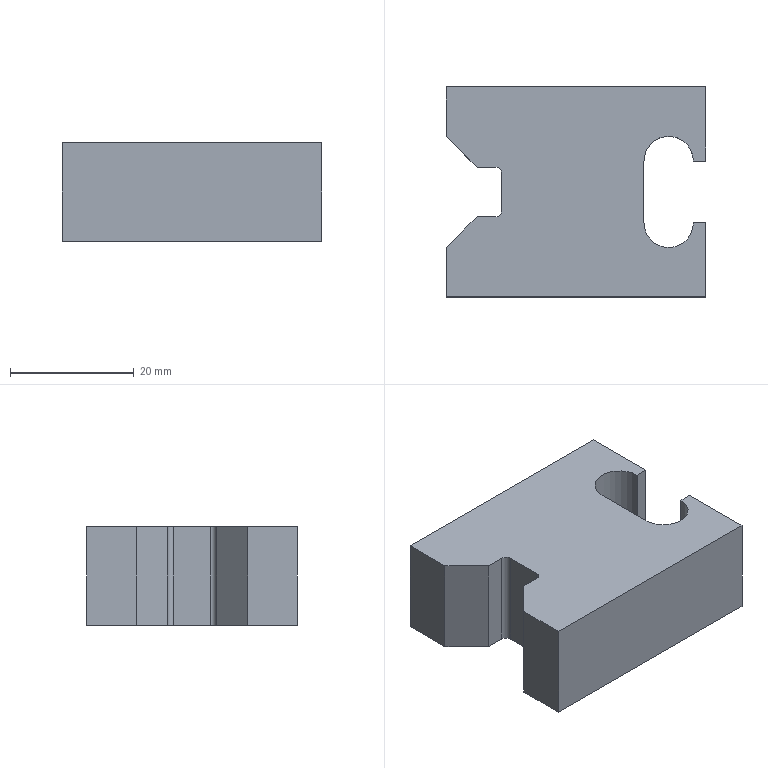Part | SolidWorks | features Cut 2, Fillet 2, Extrusion 1, ICE 1 | 1 solid | 20 faces | box 42 x 34 x 16 mm | volume 18899 mm3 | plane 16 | cylinder 4 | commonest cylinder face diameters 2 x2 8 x2
STEP:
#1=CARTESIAN_POINT('',(60.,5.,16.));
#2=VERTEX_POINT('',#1);
#3=CARTESIAN_POINT('',(60.,17.,16.));
#4=VERTEX_POINT('',#3);
#5=CARTESIAN_POINT('',(60.,17.,16.));
#6=DIRECTION('',(0.,1.,0.));
#7=VECTOR('',#6,1000.);
#8=LINE('',#5,#7);
#9=EDGE_CURVE('',#2,#4,#8,.T.);
#10=ORIENTED_EDGE('',*,*,#9,.F.);
#11=CARTESIAN_POINT('',(60.,5.,0.));
#12=VERTEX_POINT('',#11);
#13=CARTESIAN_POINT('',(60.,5.,0.));
#14=DIRECTION('',(0.,0.,1.));
#15=VECTOR('',#14,1000.);
#16=LINE('',#13,#15);
#17=EDGE_CURVE('',#12,#2,#16,.T.);
#18=ORIENTED_EDGE('',*,*,#17,.F.);
#19=CARTESIAN_POINT('',(60.,17.,0.));
#20=VERTEX_POINT('',#19);
#21=CARTESIAN_POINT('',(60.,17.,0.));
#22=DIRECTION('',(0.,1.,0.));
#23=VECTOR('',#22,1000.);
#24=LINE('',#21,#23);
#25=EDGE_CURVE('',#12,#20,#24,.T.);
#26=ORIENTED_EDGE('',*,*,#25,.T.);
#27=CARTESIAN_POINT('',(60.,17.,16.));
#28=DIRECTION('',(0.,0.,-1.));
#29=VECTOR('',#28,1000.);
#30=LINE('',#27,#29);
#31=EDGE_CURVE('',#4,#20,#30,.T.);
#32=ORIENTED_EDGE('',*,*,#31,.F.);
#33=EDGE_LOOP('',(#10,#18,#26,#32));
#34=FACE_OUTER_BOUND('',#33,.T.);
#35=CARTESIAN_POINT('',(60.,17.,16.));
#36=DIRECTION('',(-1.,0.,0.));
#37=DIRECTION('',(0.,-1.,0.));
#38=AXIS2_PLACEMENT_3D('',#35,#36,#37);
#39=PLANE('',#38);
#40=ADVANCED_FACE('',(#34),#39,.F.);
#41=CARTESIAN_POINT('',(18.,17.,0.));
#42=VERTEX_POINT('',#41);
#43=CARTESIAN_POINT('',(15.,17.,0.));
#44=DIRECTION('',(-1.,0.,0.));
#45=VECTOR('',#44,1000.);
#46=LINE('',#43,#45);
#47=EDGE_CURVE('',#20,#42,#46,.T.);
#48=ORIENTED_EDGE('',*,*,#47,.T.);
#49=CARTESIAN_POINT('',(18.,17.,16.));
#50=VERTEX_POINT('',#49);
#51=CARTESIAN_POINT('',(18.,17.,0.));
#52=DIRECTION('',(0.,0.,1.));
#53=VECTOR('',#52,1000.);
#54=LINE('',#51,#53);
#55=EDGE_CURVE('',#42,#50,#54,.T.);
#56=ORIENTED_EDGE('',*,*,#55,.T.);
#57=CARTESIAN_POINT('',(15.,17.,16.));
#58=DIRECTION('',(-1.,0.,0.));
#59=VECTOR('',#58,1000.);
#60=LINE('',#57,#59);
#61=EDGE_CURVE('',#4,#50,#60,.T.);
#62=ORIENTED_EDGE('',*,*,#61,.F.);
#63=ORIENTED_EDGE('',*,*,#31,.T.);
#64=EDGE_LOOP('',(#48,#56,#62,#63));
#65=FACE_OUTER_BOUND('',#64,.T.);
#66=CARTESIAN_POINT('',(15.,17.,16.));
#67=DIRECTION('',(0.,-1.,0.));
#68=DIRECTION('',(0.,0.,-1.));
#69=AXIS2_PLACEMENT_3D('',#66,#67,#68);
#70=PLANE('',#69);
#71=ADVANCED_FACE('',(#65),#70,.F.);
#72=CARTESIAN_POINT('',(18.,-17.,16.));
#73=VERTEX_POINT('',#72);
#74=CARTESIAN_POINT('',(60.,-17.,16.));
#75=VERTEX_POINT('',#74);
#76=CARTESIAN_POINT('',(60.,-17.,16.));
#77=DIRECTION('',(1.,0.,0.));
#78=VECTOR('',#77,1000.);
#79=LINE('',#76,#78);
#80=EDGE_CURVE('',#73,#75,#79,.T.);
#81=ORIENTED_EDGE('',*,*,#80,.F.);
#82=CARTESIAN_POINT('',(18.,-17.,0.));
#83=VERTEX_POINT('',#82);
#84=CARTESIAN_POINT('',(18.,-17.,0.));
#85=DIRECTION('',(0.,0.,1.));
#86=VECTOR('',#85,1000.);
#87=LINE('',#84,#86);
#88=EDGE_CURVE('',#83,#73,#87,.T.);
#89=ORIENTED_EDGE('',*,*,#88,.F.);
#90=CARTESIAN_POINT('',(60.,-17.,0.));
#91=VERTEX_POINT('',#90);
#92=CARTESIAN_POINT('',(60.,-17.,0.));
#93=DIRECTION('',(1.,0.,0.));
#94=VECTOR('',#93,1000.);
#95=LINE('',#92,#94);
#96=EDGE_CURVE('',#83,#91,#95,.T.);
#97=ORIENTED_EDGE('',*,*,#96,.T.);
#98=CARTESIAN_POINT('',(60.,-17.,16.));
#99=DIRECTION('',(0.,0.,-1.));
#100=VECTOR('',#99,1000.);
#101=LINE('',#98,#100);
#102=EDGE_CURVE('',#75,#91,#101,.T.);
#103=ORIENTED_EDGE('',*,*,#102,.F.);
#104=EDGE_LOOP('',(#81,#89,#97,#103));
#105=FACE_OUTER_BOUND('',#104,.T.);
#106=CARTESIAN_POINT('',(60.,-17.,16.));
#107=DIRECTION('',(0.,1.,0.));
#108=DIRECTION('',(-1.,0.,0.));
#109=AXIS2_PLACEMENT_3D('',#106,#107,#108);
#110=PLANE('',#109);
#111=ADVANCED_FACE('',(#105),#110,.F.);
#112=CARTESIAN_POINT('',(60.,-5.,0.));
#113=VERTEX_POINT('',#112);
#114=CARTESIAN_POINT('',(60.,17.,0.));
#115=DIRECTION('',(0.,1.,0.));
#116=VECTOR('',#115,1000.);
#117=LINE('',#114,#116);
#118=EDGE_CURVE('',#91,#113,#117,.T.);
#119=ORIENTED_EDGE('',*,*,#118,.T.);
#120=CARTESIAN_POINT('',(60.,-5.,16.));
#121=VERTEX_POINT('',#120);
#122=CARTESIAN_POINT('',(60.,-5.,0.));
#123=DIRECTION('',(0.,0.,1.));
#124=VECTOR('',#123,1000.);
#125=LINE('',#122,#124);
#126=EDGE_CURVE('',#113,#121,#125,.T.);
#127=ORIENTED_EDGE('',*,*,#126,.T.);
#128=CARTESIAN_POINT('',(60.,17.,16.));
#129=DIRECTION('',(0.,1.,0.));
#130=VECTOR('',#129,1000.);
#131=LINE('',#128,#130);
#132=EDGE_CURVE('',#75,#121,#131,.T.);
#133=ORIENTED_EDGE('',*,*,#132,.F.);
#134=ORIENTED_EDGE('',*,*,#102,.T.);
#135=EDGE_LOOP('',(#119,#127,#133,#134));
#136=FACE_OUTER_BOUND('',#135,.T.);
#137=CARTESIAN_POINT('',(60.,17.,16.));
#138=DIRECTION('',(-1.,0.,0.));
#139=DIRECTION('',(0.,-1.,0.));
#140=AXIS2_PLACEMENT_3D('',#137,#138,#139);
#141=PLANE('',#140);
#142=ADVANCED_FACE('',(#136),#141,.F.);
#143=CARTESIAN_POINT('',(18.,-9.,16.));
#144=VERTEX_POINT('',#143);
#145=CARTESIAN_POINT('',(18.,17.,16.));
#146=DIRECTION('',(0.,1.,0.));
#147=VECTOR('',#146,1000.);
#148=LINE('',#145,#147);
#149=EDGE_CURVE('',#73,#144,#148,.T.);
#150=ORIENTED_EDGE('',*,*,#149,.F.);
#151=ORIENTED_EDGE('',*,*,#80,.T.);
#152=ORIENTED_EDGE('',*,*,#132,.T.);
#153=CARTESIAN_POINT('',(58.,-5.,16.));
#154=VERTEX_POINT('',#153);
#155=CARTESIAN_POINT('',(58.,-5.,16.));
#156=DIRECTION('',(1.,0.,0.));
#157=VECTOR('',#156,1000.);
#158=LINE('',#155,#157);
#159=EDGE_CURVE('',#154,#121,#158,.T.);
#160=ORIENTED_EDGE('',*,*,#159,.F.);
#161=CARTESIAN_POINT('',(50.,-5.,16.));
#162=VERTEX_POINT('',#161);
#163=CARTESIAN_POINT('',(54.,-5.,16.));
#164=DIRECTION('',(0.,0.,1.));
#165=DIRECTION('',(1.,0.,0.));
#166=AXIS2_PLACEMENT_3D('',#163,#164,#165);
#167=CIRCLE('',#166,4.);
#168=EDGE_CURVE('',#162,#154,#167,.T.);
#169=ORIENTED_EDGE('',*,*,#168,.F.);
#170=CARTESIAN_POINT('',(50.,5.,16.));
#171=VERTEX_POINT('',#170);
#172=CARTESIAN_POINT('',(50.,5.,16.));
#173=DIRECTION('',(0.,-1.,0.));
#174=VECTOR('',#173,1000.);
#175=LINE('',#172,#174);
#176=EDGE_CURVE('',#171,#162,#175,.T.);
#177=ORIENTED_EDGE('',*,*,#176,.F.);
#178=CARTESIAN_POINT('',(58.,5.,16.));
#179=VERTEX_POINT('',#178);
#180=CARTESIAN_POINT('',(54.,5.,16.));
#181=DIRECTION('',(0.,0.,1.));
#182=DIRECTION('',(-1.,0.,0.));
#183=AXIS2_PLACEMENT_3D('',#180,#181,#182);
#184=CIRCLE('',#183,4.);
#185=EDGE_CURVE('',#179,#171,#184,.T.);
#186=ORIENTED_EDGE('',*,*,#185,.F.);
#187=CARTESIAN_POINT('',(58.,5.,16.));
#188=DIRECTION('',(-1.,0.,0.));
#189=VECTOR('',#188,1000.);
#190=LINE('',#187,#189);
#191=EDGE_CURVE('',#2,#179,#190,.T.);
#192=ORIENTED_EDGE('',*,*,#191,.F.);
#193=ORIENTED_EDGE('',*,*,#9,.T.);
#194=ORIENTED_EDGE('',*,*,#61,.T.);
#195=CARTESIAN_POINT('',(18.,9.,16.));
#196=VERTEX_POINT('',#195);
#197=CARTESIAN_POINT('',(18.,17.,16.));
#198=DIRECTION('',(0.,1.,0.));
#199=VECTOR('',#198,1000.);
#200=LINE('',#197,#199);
#201=EDGE_CURVE('',#196,#50,#200,.T.);
#202=ORIENTED_EDGE('',*,*,#201,.F.);
#203=CARTESIAN_POINT('',(23.,4.,16.));
#204=VERTEX_POINT('',#203);
#205=CARTESIAN_POINT('',(23.,4.,16.));
#206=DIRECTION('',(-0.7071,0.7071,0.));
#207=VECTOR('',#206,1000.);
#208=LINE('',#205,#207);
#209=EDGE_CURVE('',#204,#196,#208,.T.);
#210=ORIENTED_EDGE('',*,*,#209,.F.);
#211=CARTESIAN_POINT('',(26.,4.,16.));
#212=VERTEX_POINT('',#211);
#213=CARTESIAN_POINT('',(27.,4.,16.));
#214=DIRECTION('',(-1.,0.,0.));
#215=VECTOR('',#214,1000.);
#216=LINE('',#213,#215);
#217=EDGE_CURVE('',#212,#204,#216,.T.);
#218=ORIENTED_EDGE('',*,*,#217,.F.);
#219=CARTESIAN_POINT('',(27.,3.,16.));
#220=VERTEX_POINT('',#219);
#221=CARTESIAN_POINT('',(26.,3.,16.));
#222=DIRECTION('',(0.,0.,-1.));
#223=DIRECTION('',(1.,0.,0.));
#224=AXIS2_PLACEMENT_3D('',#221,#222,#223);
#225=CIRCLE('',#224,1.);
#226=EDGE_CURVE('',#212,#220,#225,.T.);
#227=ORIENTED_EDGE('',*,*,#226,.T.);
#228=CARTESIAN_POINT('',(27.,-3.,16.));
#229=VERTEX_POINT('',#228);
#230=CARTESIAN_POINT('',(27.,4.,16.));
#231=DIRECTION('',(0.,1.,0.));
#232=VECTOR('',#231,1000.);
#233=LINE('',#230,#232);
#234=EDGE_CURVE('',#229,#220,#233,.T.);
#235=ORIENTED_EDGE('',*,*,#234,.F.);
#236=CARTESIAN_POINT('',(26.,-4.,16.));
#237=VERTEX_POINT('',#236);
#238=CARTESIAN_POINT('',(26.,-3.,16.));
#239=DIRECTION('',(0.,0.,-1.));
#240=DIRECTION('',(1.,0.,0.));
#241=AXIS2_PLACEMENT_3D('',#238,#239,#240);
#242=CIRCLE('',#241,1.);
#243=EDGE_CURVE('',#229,#237,#242,.T.);
#244=ORIENTED_EDGE('',*,*,#243,.T.);
#245=CARTESIAN_POINT('',(23.,-4.,16.));
#246=VERTEX_POINT('',#245);
#247=CARTESIAN_POINT('',(27.,-4.,16.));
#248=DIRECTION('',(1.,0.,0.));
#249=VECTOR('',#248,1000.);
#250=LINE('',#247,#249);
#251=EDGE_CURVE('',#246,#237,#250,.T.);
#252=ORIENTED_EDGE('',*,*,#251,.F.);
#253=CARTESIAN_POINT('',(23.,-4.,16.));
#254=DIRECTION('',(0.7071,0.7071,0.));
#255=VECTOR('',#254,1000.);
#256=LINE('',#253,#255);
#257=EDGE_CURVE('',#144,#246,#256,.T.);
#258=ORIENTED_EDGE('',*,*,#257,.F.);
#259=EDGE_LOOP('',(#150,#151,#152,#160,#169,#177,#186,#192,#193,#194,#202,#210,#218,#227,#235,#244,#252,#258));
#260=FACE_OUTER_BOUND('',#259,.T.);
#261=CARTESIAN_POINT('',(15.,17.,16.));
#262=DIRECTION('',(0.,0.,1.));
#263=DIRECTION('',(1.,0.,0.));
#264=AXIS2_PLACEMENT_3D('',#261,#262,#263);
#265=PLANE('',#264);
#266=ADVANCED_FACE('',(#260),#265,.T.);
#267=ORIENTED_EDGE('',*,*,#96,.F.);
#268=CARTESIAN_POINT('',(18.,-9.,0.));
#269=VERTEX_POINT('',#268);
#270=CARTESIAN_POINT('',(18.,17.,0.));
#271=DIRECTION('',(0.,1.,0.));
#272=VECTOR('',#271,1000.);
#273=LINE('',#270,#272);
#274=EDGE_CURVE('',#83,#269,#273,.T.);
#275=ORIENTED_EDGE('',*,*,#274,.T.);
#276=CARTESIAN_POINT('',(23.,-4.,0.));
#277=VERTEX_POINT('',#276);
#278=CARTESIAN_POINT('',(23.,-4.,0.));
#279=DIRECTION('',(0.7071,0.7071,0.));
#280=VECTOR('',#279,1000.);
#281=LINE('',#278,#280);
#282=EDGE_CURVE('',#269,#277,#281,.T.);
#283=ORIENTED_EDGE('',*,*,#282,.T.);
#284=CARTESIAN_POINT('',(26.,-4.,0.));
#285=VERTEX_POINT('',#284);
#286=CARTESIAN_POINT('',(27.,-4.,0.));
#287=DIRECTION('',(1.,0.,0.));
#288=VECTOR('',#287,1000.);
#289=LINE('',#286,#288);
#290=EDGE_CURVE('',#277,#285,#289,.T.);
#291=ORIENTED_EDGE('',*,*,#290,.T.);
#292=CARTESIAN_POINT('',(27.,-3.,0.));
#293=VERTEX_POINT('',#292);
#294=CARTESIAN_POINT('',(26.,-3.,0.));
#295=DIRECTION('',(0.,0.,1.));
#296=DIRECTION('',(1.,0.,0.));
#297=AXIS2_PLACEMENT_3D('',#294,#295,#296);
#298=CIRCLE('',#297,1.);
#299=EDGE_CURVE('',#285,#293,#298,.T.);
#300=ORIENTED_EDGE('',*,*,#299,.T.);
#301=CARTESIAN_POINT('',(27.,3.,0.));
#302=VERTEX_POINT('',#301);
#303=CARTESIAN_POINT('',(27.,4.,0.));
#304=DIRECTION('',(0.,1.,0.));
#305=VECTOR('',#304,1000.);
#306=LINE('',#303,#305);
#307=EDGE_CURVE('',#293,#302,#306,.T.);
#308=ORIENTED_EDGE('',*,*,#307,.T.);
#309=CARTESIAN_POINT('',(26.,4.,0.));
#310=VERTEX_POINT('',#309);
#311=CARTESIAN_POINT('',(26.,3.,0.));
#312=DIRECTION('',(0.,0.,1.));
#313=DIRECTION('',(1.,0.,0.));
#314=AXIS2_PLACEMENT_3D('',#311,#312,#313);
#315=CIRCLE('',#314,1.);
#316=EDGE_CURVE('',#302,#310,#315,.T.);
#317=ORIENTED_EDGE('',*,*,#316,.T.);
#318=CARTESIAN_POINT('',(23.,4.,0.));
#319=VERTEX_POINT('',#318);
#320=CARTESIAN_POINT('',(27.,4.,0.));
#321=DIRECTION('',(-1.,0.,0.));
#322=VECTOR('',#321,1000.);
#323=LINE('',#320,#322);
#324=EDGE_CURVE('',#310,#319,#323,.T.);
#325=ORIENTED_EDGE('',*,*,#324,.T.);
#326=CARTESIAN_POINT('',(18.,9.,0.));
#327=VERTEX_POINT('',#326);
#328=CARTESIAN_POINT('',(23.,4.,0.));
#329=DIRECTION('',(-0.7071,0.7071,0.));
#330=VECTOR('',#329,1000.);
#331=LINE('',#328,#330);
#332=EDGE_CURVE('',#319,#327,#331,.T.);
#333=ORIENTED_EDGE('',*,*,#332,.T.);
#334=CARTESIAN_POINT('',(18.,17.,0.));
#335=DIRECTION('',(0.,1.,0.));
#336=VECTOR('',#335,1000.);
#337=LINE('',#334,#336);
#338=EDGE_CURVE('',#327,#42,#337,.T.);
#339=ORIENTED_EDGE('',*,*,#338,.T.);
#340=ORIENTED_EDGE('',*,*,#47,.F.);
#341=ORIENTED_EDGE('',*,*,#25,.F.);
#342=CARTESIAN_POINT('',(58.,5.,0.));
#343=VERTEX_POINT('',#342);
#344=CARTESIAN_POINT('',(58.,5.,0.));
#345=DIRECTION('',(-1.,0.,0.));
#346=VECTOR('',#345,1000.);
#347=LINE('',#344,#346);
#348=EDGE_CURVE('',#12,#343,#347,.T.);
#349=ORIENTED_EDGE('',*,*,#348,.T.);
#350=CARTESIAN_POINT('',(50.,5.,0.));
#351=VERTEX_POINT('',#350);
#352=CARTESIAN_POINT('',(54.,5.,0.));
#353=DIRECTION('',(0.,0.,1.));
#354=DIRECTION('',(-1.,0.,0.));
#355=AXIS2_PLACEMENT_3D('',#352,#353,#354);
#356=CIRCLE('',#355,4.);
#357=EDGE_CURVE('',#343,#351,#356,.T.);
#358=ORIENTED_EDGE('',*,*,#357,.T.);
#359=CARTESIAN_POINT('',(50.,-5.,0.));
#360=VERTEX_POINT('',#359);
#361=CARTESIAN_POINT('',(50.,5.,0.));
#362=DIRECTION('',(0.,-1.,0.));
#363=VECTOR('',#362,1000.);
#364=LINE('',#361,#363);
#365=EDGE_CURVE('',#351,#360,#364,.T.);
#366=ORIENTED_EDGE('',*,*,#365,.T.);
#367=CARTESIAN_POINT('',(58.,-5.,0.));
#368=VERTEX_POINT('',#367);
#369=CARTESIAN_POINT('',(54.,-5.,0.));
#370=DIRECTION('',(0.,0.,1.));
#371=DIRECTION('',(1.,0.,0.));
#372=AXIS2_PLACEMENT_3D('',#369,#370,#371);
#373=CIRCLE('',#372,4.);
#374=EDGE_CURVE('',#360,#368,#373,.T.);
#375=ORIENTED_EDGE('',*,*,#374,.T.);
#376=CARTESIAN_POINT('',(58.,-5.,0.));
#377=DIRECTION('',(1.,0.,0.));
#378=VECTOR('',#377,1000.);
#379=LINE('',#376,#378);
#380=EDGE_CURVE('',#368,#113,#379,.T.);
#381=ORIENTED_EDGE('',*,*,#380,.T.);
#382=ORIENTED_EDGE('',*,*,#118,.F.);
#383=EDGE_LOOP('',(#267,#275,#283,#291,#300,#308,#317,#325,#333,#339,#340,#341,#349,#358,#366,#375,#381,#382));
#384=FACE_OUTER_BOUND('',#383,.T.);
#385=CARTESIAN_POINT('',(15.,17.,0.));
#386=DIRECTION('',(0.,0.,1.));
#387=DIRECTION('',(1.,0.,0.));
#388=AXIS2_PLACEMENT_3D('',#385,#386,#387);
#389=PLANE('',#388);
#390=ADVANCED_FACE('',(#384),#389,.F.);
#391=ORIENTED_EDGE('',*,*,#324,.F.);
#392=CARTESIAN_POINT('',(26.,4.,16.));
#393=DIRECTION('',(0.,0.,1.));
#394=VECTOR('',#393,1000.);
#395=LINE('',#392,#394);
#396=EDGE_CURVE('',#310,#212,#395,.T.);
#397=ORIENTED_EDGE('',*,*,#396,.T.);
#398=ORIENTED_EDGE('',*,*,#217,.T.);
#399=CARTESIAN_POINT('',(23.,4.,0.));
#400=DIRECTION('',(0.,0.,1.));
#401=VECTOR('',#400,1000.);
#402=LINE('',#399,#401);
#403=EDGE_CURVE('',#319,#204,#402,.T.);
#404=ORIENTED_EDGE('',*,*,#403,.F.);
#405=EDGE_LOOP('',(#391,#397,#398,#404));
#406=FACE_OUTER_BOUND('',#405,.T.);
#407=CARTESIAN_POINT('',(27.,4.,0.));
#408=DIRECTION('',(0.,1.,0.));
#409=DIRECTION('',(0.,0.,1.));
#410=AXIS2_PLACEMENT_3D('',#407,#408,#409);
#411=PLANE('',#410);
#412=ADVANCED_FACE('',(#406),#411,.F.);
#413=ORIENTED_EDGE('',*,*,#307,.F.);
#414=CARTESIAN_POINT('',(27.,-3.,16.));
#415=DIRECTION('',(0.,0.,1.));
#416=VECTOR('',#415,1000.);
#417=LINE('',#414,#416);
#418=EDGE_CURVE('',#293,#229,#417,.T.);
#419=ORIENTED_EDGE('',*,*,#418,.T.);
#420=ORIENTED_EDGE('',*,*,#234,.T.);
#421=CARTESIAN_POINT('',(27.,3.,0.));
#422=DIRECTION('',(0.,0.,-1.));
#423=VECTOR('',#422,1000.);
#424=LINE('',#421,#423);
#425=EDGE_CURVE('',#220,#302,#424,.T.);
#426=ORIENTED_EDGE('',*,*,#425,.T.);
#427=EDGE_LOOP('',(#413,#419,#420,#426));
#428=FACE_OUTER_BOUND('',#427,.T.);
#429=CARTESIAN_POINT('',(27.,4.,0.));
#430=DIRECTION('',(1.,0.,0.));
#431=DIRECTION('',(0.,0.,-1.));
#432=AXIS2_PLACEMENT_3D('',#429,#430,#431);
#433=PLANE('',#432);
#434=ADVANCED_FACE('',(#428),#433,.F.);
#435=ORIENTED_EDGE('',*,*,#251,.T.);
#436=CARTESIAN_POINT('',(26.,-4.,0.));
#437=DIRECTION('',(0.,0.,-1.));
#438=VECTOR('',#437,1000.);
#439=LINE('',#436,#438);
#440=EDGE_CURVE('',#237,#285,#439,.T.);
#441=ORIENTED_EDGE('',*,*,#440,.T.);
#442=ORIENTED_EDGE('',*,*,#290,.F.);
#443=CARTESIAN_POINT('',(23.,-4.,0.));
#444=DIRECTION('',(0.,0.,1.));
#445=VECTOR('',#444,1000.);
#446=LINE('',#443,#445);
#447=EDGE_CURVE('',#277,#246,#446,.T.);
#448=ORIENTED_EDGE('',*,*,#447,.T.);
#449=EDGE_LOOP('',(#435,#441,#442,#448));
#450=FACE_OUTER_BOUND('',#449,.T.);
#451=CARTESIAN_POINT('',(27.,-4.,0.));
#452=DIRECTION('',(0.,-1.,0.));
#453=DIRECTION('',(1.,0.,0.));
#454=AXIS2_PLACEMENT_3D('',#451,#452,#453);
#455=PLANE('',#454);
#456=ADVANCED_FACE('',(#450),#455,.F.);
#457=ORIENTED_EDGE('',*,*,#282,.F.);
#458=CARTESIAN_POINT('',(18.,-9.,0.));
#459=DIRECTION('',(0.,0.,1.));
#460=VECTOR('',#459,1000.);
#461=LINE('',#458,#460);
#462=EDGE_CURVE('',#269,#144,#461,.T.);
#463=ORIENTED_EDGE('',*,*,#462,.T.);
#464=ORIENTED_EDGE('',*,*,#257,.T.);
#465=ORIENTED_EDGE('',*,*,#447,.F.);
#466=EDGE_LOOP('',(#457,#463,#464,#465));
#467=FACE_OUTER_BOUND('',#466,.T.);
#468=CARTESIAN_POINT('',(23.,-4.,0.));
#469=DIRECTION('',(0.7071,-0.7071,0.));
#470=DIRECTION('',(0.7071,0.7071,0.));
#471=AXIS2_PLACEMENT_3D('',#468,#469,#470);
#472=PLANE('',#471);
#473=ADVANCED_FACE('',(#467),#472,.F.);
#474=ORIENTED_EDGE('',*,*,#209,.T.);
#475=CARTESIAN_POINT('',(18.,9.,0.));
#476=DIRECTION('',(0.,0.,-1.));
#477=VECTOR('',#476,1000.);
#478=LINE('',#475,#477);
#479=EDGE_CURVE('',#196,#327,#478,.T.);
#480=ORIENTED_EDGE('',*,*,#479,.T.);
#481=ORIENTED_EDGE('',*,*,#332,.F.);
#482=ORIENTED_EDGE('',*,*,#403,.T.);
#483=EDGE_LOOP('',(#474,#480,#481,#482));
#484=FACE_OUTER_BOUND('',#483,.T.);
#485=CARTESIAN_POINT('',(23.,4.,0.));
#486=DIRECTION('',(0.7071,0.7071,0.));
#487=DIRECTION('',(-0.7071,0.7071,0.));
#488=AXIS2_PLACEMENT_3D('',#485,#486,#487);
#489=PLANE('',#488);
#490=ADVANCED_FACE('',(#484),#489,.F.);
#491=ORIENTED_EDGE('',*,*,#316,.F.);
#492=ORIENTED_EDGE('',*,*,#425,.F.);
#493=ORIENTED_EDGE('',*,*,#226,.F.);
#494=ORIENTED_EDGE('',*,*,#396,.F.);
#495=EDGE_LOOP('',(#491,#492,#493,#494));
#496=FACE_OUTER_BOUND('',#495,.T.);
#497=CARTESIAN_POINT('',(26.,3.,0.));
#498=DIRECTION('',(0.,0.,-1.));
#499=DIRECTION('',(-1.,0.,0.));
#500=AXIS2_PLACEMENT_3D('',#497,#498,#499);
#501=CYLINDRICAL_SURFACE('',#500,1.);
#502=ADVANCED_FACE('',(#496),#501,.F.);
#503=ORIENTED_EDGE('',*,*,#299,.F.);
#504=ORIENTED_EDGE('',*,*,#440,.F.);
#505=ORIENTED_EDGE('',*,*,#243,.F.);
#506=ORIENTED_EDGE('',*,*,#418,.F.);
#507=EDGE_LOOP('',(#503,#504,#505,#506));
#508=FACE_OUTER_BOUND('',#507,.T.);
#509=CARTESIAN_POINT('',(26.,-3.,0.));
#510=DIRECTION('',(0.,0.,-1.));
#511=DIRECTION('',(-1.,0.,0.));
#512=AXIS2_PLACEMENT_3D('',#509,#510,#511);
#513=CYLINDRICAL_SURFACE('',#512,1.);
#514=ADVANCED_FACE('',(#508),#513,.F.);
#515=ORIENTED_EDGE('',*,*,#185,.T.);
#516=CARTESIAN_POINT('',(50.,5.,0.));
#517=DIRECTION('',(0.,0.,1.));
#518=VECTOR('',#517,1000.);
#519=LINE('',#516,#518);
#520=EDGE_CURVE('',#351,#171,#519,.T.);
#521=ORIENTED_EDGE('',*,*,#520,.F.);
#522=ORIENTED_EDGE('',*,*,#357,.F.);
#523=CARTESIAN_POINT('',(58.,5.,0.));
#524=DIRECTION('',(0.,0.,1.));
#525=VECTOR('',#524,1000.);
#526=LINE('',#523,#525);
#527=EDGE_CURVE('',#343,#179,#526,.T.);
#528=ORIENTED_EDGE('',*,*,#527,.T.);
#529=EDGE_LOOP('',(#515,#521,#522,#528));
#530=FACE_OUTER_BOUND('',#529,.T.);
#531=CARTESIAN_POINT('',(54.,5.,0.));
#532=DIRECTION('',(0.,0.,1.));
#533=DIRECTION('',(1.,0.,0.));
#534=AXIS2_PLACEMENT_3D('',#531,#532,#533);
#535=CYLINDRICAL_SURFACE('',#534,4.);
#536=ADVANCED_FACE('',(#530),#535,.F.);
#537=ORIENTED_EDGE('',*,*,#191,.T.);
#538=ORIENTED_EDGE('',*,*,#527,.F.);
#539=ORIENTED_EDGE('',*,*,#348,.F.);
#540=ORIENTED_EDGE('',*,*,#17,.T.);
#541=EDGE_LOOP('',(#537,#538,#539,#540));
#542=FACE_OUTER_BOUND('',#541,.T.);
#543=CARTESIAN_POINT('',(58.,5.,0.));
#544=DIRECTION('',(0.,1.,0.));
#545=DIRECTION('',(0.,0.,1.));
#546=AXIS2_PLACEMENT_3D('',#543,#544,#545);
#547=PLANE('',#546);
#548=ADVANCED_FACE('',(#542),#547,.F.);
#549=ORIENTED_EDGE('',*,*,#159,.T.);
#550=ORIENTED_EDGE('',*,*,#126,.F.);
#551=ORIENTED_EDGE('',*,*,#380,.F.);
#552=CARTESIAN_POINT('',(58.,-5.,0.));
#553=DIRECTION('',(0.,0.,1.));
#554=VECTOR('',#553,1000.);
#555=LINE('',#552,#554);
#556=EDGE_CURVE('',#368,#154,#555,.T.);
#557=ORIENTED_EDGE('',*,*,#556,.T.);
#558=EDGE_LOOP('',(#549,#550,#551,#557));
#559=FACE_OUTER_BOUND('',#558,.T.);
#560=CARTESIAN_POINT('',(58.,-5.,0.));
#561=DIRECTION('',(0.,-1.,0.));
#562=DIRECTION('',(0.,0.,-1.));
#563=AXIS2_PLACEMENT_3D('',#560,#561,#562);
#564=PLANE('',#563);
#565=ADVANCED_FACE('',(#559),#564,.F.);
#566=ORIENTED_EDGE('',*,*,#168,.T.);
#567=ORIENTED_EDGE('',*,*,#556,.F.);
#568=ORIENTED_EDGE('',*,*,#374,.F.);
#569=CARTESIAN_POINT('',(50.,-5.,0.));
#570=DIRECTION('',(0.,0.,1.));
#571=VECTOR('',#570,1000.);
#572=LINE('',#569,#571);
#573=EDGE_CURVE('',#360,#162,#572,.T.);
#574=ORIENTED_EDGE('',*,*,#573,.T.);
#575=EDGE_LOOP('',(#566,#567,#568,#574));
#576=FACE_OUTER_BOUND('',#575,.T.);
#577=CARTESIAN_POINT('',(54.,-5.,0.));
#578=DIRECTION('',(0.,0.,1.));
#579=DIRECTION('',(1.,0.,0.));
#580=AXIS2_PLACEMENT_3D('',#577,#578,#579);
#581=CYLINDRICAL_SURFACE('',#580,4.);
#582=ADVANCED_FACE('',(#576),#581,.F.);
#583=ORIENTED_EDGE('',*,*,#176,.T.);
#584=ORIENTED_EDGE('',*,*,#573,.F.);
#585=ORIENTED_EDGE('',*,*,#365,.F.);
#586=ORIENTED_EDGE('',*,*,#520,.T.);
#587=EDGE_LOOP('',(#583,#584,#585,#586));
#588=FACE_OUTER_BOUND('',#587,.T.);
#589=CARTESIAN_POINT('',(50.,5.,0.));
#590=DIRECTION('',(-1.,0.,0.));
#591=DIRECTION('',(0.,-1.,0.));
#592=AXIS2_PLACEMENT_3D('',#589,#590,#591);
#593=PLANE('',#592);
#594=ADVANCED_FACE('',(#588),#593,.F.);
#595=ORIENTED_EDGE('',*,*,#201,.T.);
#596=ORIENTED_EDGE('',*,*,#55,.F.);
#597=ORIENTED_EDGE('',*,*,#338,.F.);
#598=ORIENTED_EDGE('',*,*,#479,.F.);
#599=EDGE_LOOP('',(#595,#596,#597,#598));
#600=FACE_OUTER_BOUND('',#599,.T.);
#601=CARTESIAN_POINT('',(18.,17.,0.));
#602=DIRECTION('',(1.,0.,0.));
#603=DIRECTION('',(0.,1.,0.));
#604=AXIS2_PLACEMENT_3D('',#601,#602,#603);
#605=PLANE('',#604);
#606=ADVANCED_FACE('',(#600),#605,.F.);
#607=ORIENTED_EDGE('',*,*,#274,.F.);
#608=ORIENTED_EDGE('',*,*,#88,.T.);
#609=ORIENTED_EDGE('',*,*,#149,.T.);
#610=ORIENTED_EDGE('',*,*,#462,.F.);
#611=EDGE_LOOP('',(#607,#608,#609,#610));
#612=FACE_OUTER_BOUND('',#611,.T.);
#613=CARTESIAN_POINT('',(18.,17.,0.));
#614=DIRECTION('',(1.,0.,0.));
#615=DIRECTION('',(0.,1.,0.));
#616=AXIS2_PLACEMENT_3D('',#613,#614,#615);
#617=PLANE('',#616);
#618=ADVANCED_FACE('',(#612),#617,.F.);
#619=CLOSED_SHELL('',(#40,#71,#111,#142,#266,#390,#412,#434,#456,#473,#490,#502,#514,#536,#548,#565,#582,#594,#606,#618));
#620=MANIFOLD_SOLID_BREP('',#619);
#621=CARTESIAN_POINT('',(0.,0.,0.));
#622=DIRECTION('',(0.,0.,1.));
#623=DIRECTION('',(1.,0.,0.));
#624=AXIS2_PLACEMENT_3D('',#621,#622,#623);
#625=(LENGTH_UNIT()NAMED_UNIT(*)SI_UNIT(.MILLI.,.METRE.));
#626=UNCERTAINTY_MEASURE_WITH_UNIT(LENGTH_MEASURE(0.00001),#625,'','');
#627=(NAMED_UNIT(*)PLANE_ANGLE_UNIT()SI_UNIT($,.RADIAN.));
#628=(NAMED_UNIT(*)SI_UNIT($,.STERADIAN.)SOLID_ANGLE_UNIT());
#629=(GEOMETRIC_REPRESENTATION_CONTEXT(3)GLOBAL_UNCERTAINTY_ASSIGNED_CONTEXT((#626))GLOBAL_UNIT_ASSIGNED_CONTEXT((#625,#627,#628))REPRESENTATION_CONTEXT('',''));
#630=ADVANCED_BREP_SHAPE_REPRESENTATION('',(#620,#624),#629);